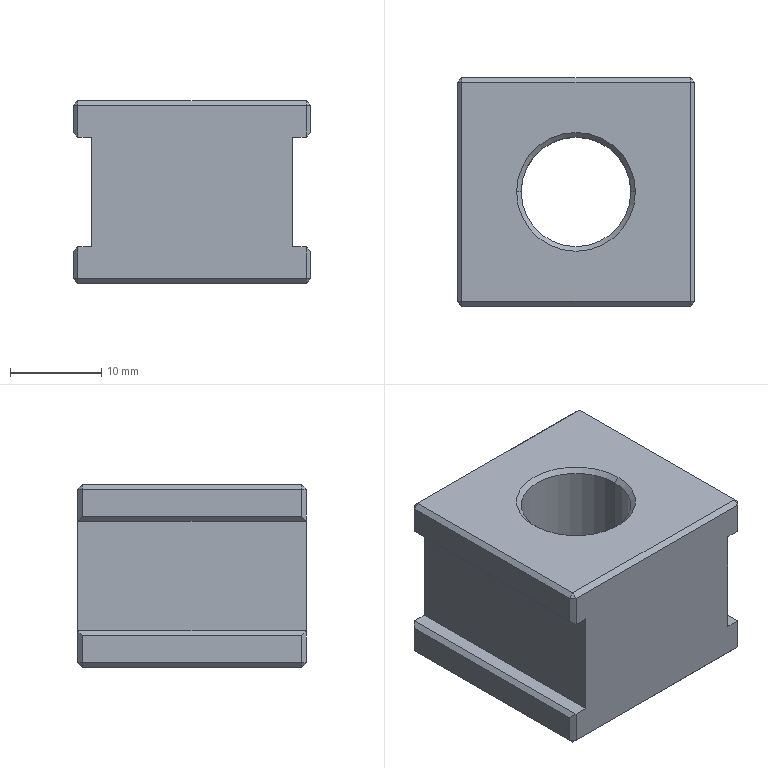Part | STEP file | MT-COMBO-119-S014 | 1 solid | 51 faces | box 26 x 25 x 20 mm | volume 9252 mm3 | plane 43 | cylinder 4 | cone 4 | commonest cylinder face diameters 10 x2 12 x2
STEP:
#1=CARTESIAN_POINT('',(0.,9.5,-15.));
#2=VERTEX_POINT('',#1);
#3=CARTESIAN_POINT('',(0.,9.5,-5.));
#4=VERTEX_POINT('',#3);
#5=CARTESIAN_POINT('',(0.,9.5,-10.));
#6=DIRECTION('',(0.,-1.,0.));
#7=DIRECTION('',(0.,0.,-1.));
#8=AXIS2_PLACEMENT_3D('',#5,#6,#7);
#9=CIRCLE('',#8,5.);
#10=EDGE_CURVE('',#2,#4,#9,.T.);
#11=ORIENTED_EDGE('',*,*,#10,.T.);
#12=CARTESIAN_POINT('',(0.,12.5,-5.));
#13=VERTEX_POINT('',#12);
#14=CARTESIAN_POINT('',(0.,9.5,-5.));
#15=DIRECTION('',(0.,1.,0.));
#16=VECTOR('',#15,1000.);
#17=LINE('',#14,#16);
#18=EDGE_CURVE('',#4,#13,#17,.T.);
#19=ORIENTED_EDGE('',*,*,#18,.T.);
#20=CARTESIAN_POINT('',(0.,12.5,-15.));
#21=VERTEX_POINT('',#20);
#22=CARTESIAN_POINT('',(0.,12.5,-10.));
#23=DIRECTION('',(0.,-1.,0.));
#24=DIRECTION('',(0.,0.,-1.));
#25=AXIS2_PLACEMENT_3D('',#22,#23,#24);
#26=CIRCLE('',#25,5.);
#27=EDGE_CURVE('',#21,#13,#26,.T.);
#28=ORIENTED_EDGE('',*,*,#27,.F.);
#29=CARTESIAN_POINT('',(0.,9.5,-15.));
#30=DIRECTION('',(0.,1.,0.));
#31=VECTOR('',#30,1000.);
#32=LINE('',#29,#31);
#33=EDGE_CURVE('',#2,#21,#32,.T.);
#34=ORIENTED_EDGE('',*,*,#33,.F.);
#35=EDGE_LOOP('',(#11,#19,#28,#34));
#36=FACE_OUTER_BOUND('',#35,.T.);
#37=CARTESIAN_POINT('',(0.,9.5,-10.));
#38=DIRECTION('',(0.,1.,0.));
#39=DIRECTION('',(0.,0.,-1.));
#40=AXIS2_PLACEMENT_3D('',#37,#38,#39);
#41=CYLINDRICAL_SURFACE('',#40,5.);
#42=ADVANCED_FACE('',(#36),#41,.F.);
#43=CARTESIAN_POINT('',(-6.,0.,-0.5));
#44=VERTEX_POINT('',#43);
#45=CARTESIAN_POINT('',(6.,0.,-0.5));
#46=VERTEX_POINT('',#45);
#47=CARTESIAN_POINT('',(0.,0.,-0.5));
#48=DIRECTION('',(0.,0.,-1.));
#49=DIRECTION('',(1.,0.,0.));
#50=AXIS2_PLACEMENT_3D('',#47,#48,#49);
#51=CIRCLE('',#50,6.);
#52=EDGE_CURVE('',#44,#46,#51,.T.);
#53=ORIENTED_EDGE('',*,*,#52,.T.);
#54=CARTESIAN_POINT('',(6.5,0.,0.));
#55=VERTEX_POINT('',#54);
#56=CARTESIAN_POINT('',(6.5,0.,0.));
#57=DIRECTION('',(0.7071,0.,0.7071));
#58=VECTOR('',#57,1000.);
#59=LINE('',#56,#58);
#60=EDGE_CURVE('',#46,#55,#59,.T.);
#61=ORIENTED_EDGE('',*,*,#60,.T.);
#62=CARTESIAN_POINT('',(-6.5,0.,0.));
#63=VERTEX_POINT('',#62);
#64=CARTESIAN_POINT('',(0.,0.,0.));
#65=DIRECTION('',(0.,0.,1.));
#66=DIRECTION('',(1.,0.,0.));
#67=AXIS2_PLACEMENT_3D('',#64,#65,#66);
#68=CIRCLE('',#67,6.5);
#69=EDGE_CURVE('',#55,#63,#68,.T.);
#70=ORIENTED_EDGE('',*,*,#69,.T.);
#71=CARTESIAN_POINT('',(-6.5,0.,0.));
#72=DIRECTION('',(-0.7071,0.,0.7071));
#73=VECTOR('',#72,1000.);
#74=LINE('',#71,#73);
#75=EDGE_CURVE('',#44,#63,#74,.T.);
#76=ORIENTED_EDGE('',*,*,#75,.F.);
#77=EDGE_LOOP('',(#53,#61,#70,#76));
#78=FACE_OUTER_BOUND('',#77,.T.);
#79=CARTESIAN_POINT('',(0.,0.,0.));
#80=DIRECTION('',(0.,0.,1.));
#81=DIRECTION('',(-1.,0.,0.));
#82=AXIS2_PLACEMENT_3D('',#79,#80,#81);
#83=CONICAL_SURFACE('',#82,6.5,0.7854);
#84=ADVANCED_FACE('',(#78),#83,.F.);
#85=CARTESIAN_POINT('',(6.,0.,-19.5));
#86=VERTEX_POINT('',#85);
#87=CARTESIAN_POINT('',(-6.,0.,-19.5));
#88=VERTEX_POINT('',#87);
#89=CARTESIAN_POINT('',(0.,0.,-19.5));
#90=DIRECTION('',(0.,0.,1.));
#91=DIRECTION('',(1.,0.,0.));
#92=AXIS2_PLACEMENT_3D('',#89,#90,#91);
#93=CIRCLE('',#92,6.);
#94=EDGE_CURVE('',#86,#88,#93,.T.);
#95=ORIENTED_EDGE('',*,*,#94,.T.);
#96=CARTESIAN_POINT('',(-6.5,0.,-20.));
#97=VERTEX_POINT('',#96);
#98=CARTESIAN_POINT('',(-6.,0.,-19.5));
#99=DIRECTION('',(-0.7071,0.,-0.7071));
#100=VECTOR('',#99,1000.);
#101=LINE('',#98,#100);
#102=EDGE_CURVE('',#88,#97,#101,.T.);
#103=ORIENTED_EDGE('',*,*,#102,.T.);
#104=CARTESIAN_POINT('',(6.5,0.,-20.));
#105=VERTEX_POINT('',#104);
#106=CARTESIAN_POINT('',(0.,0.,-20.));
#107=DIRECTION('',(0.,0.,-1.));
#108=DIRECTION('',(1.,0.,0.));
#109=AXIS2_PLACEMENT_3D('',#106,#107,#108);
#110=CIRCLE('',#109,6.5);
#111=EDGE_CURVE('',#97,#105,#110,.T.);
#112=ORIENTED_EDGE('',*,*,#111,.T.);
#113=CARTESIAN_POINT('',(6.,0.,-19.5));
#114=DIRECTION('',(0.7071,0.,-0.7071));
#115=VECTOR('',#114,1000.);
#116=LINE('',#113,#115);
#117=EDGE_CURVE('',#86,#105,#116,.T.);
#118=ORIENTED_EDGE('',*,*,#117,.F.);
#119=EDGE_LOOP('',(#95,#103,#112,#118));
#120=FACE_OUTER_BOUND('',#119,.T.);
#121=CARTESIAN_POINT('',(0.,0.,-19.5));
#122=DIRECTION('',(0.,0.,-1.));
#123=DIRECTION('',(1.,0.,0.));
#124=AXIS2_PLACEMENT_3D('',#121,#122,#123);
#125=CONICAL_SURFACE('',#124,6.,0.7854);
#126=ADVANCED_FACE('',(#120),#125,.F.);
#127=ORIENTED_EDGE('',*,*,#52,.F.);
#128=CARTESIAN_POINT('',(-6.,0.,0.));
#129=DIRECTION('',(0.,0.,-1.));
#130=VECTOR('',#129,1000.);
#131=LINE('',#128,#130);
#132=EDGE_CURVE('',#44,#88,#131,.T.);
#133=ORIENTED_EDGE('',*,*,#132,.T.);
#134=ORIENTED_EDGE('',*,*,#94,.F.);
#135=CARTESIAN_POINT('',(6.,0.,0.));
#136=DIRECTION('',(0.,0.,-1.));
#137=VECTOR('',#136,1000.);
#138=LINE('',#135,#137);
#139=EDGE_CURVE('',#46,#86,#138,.T.);
#140=ORIENTED_EDGE('',*,*,#139,.F.);
#141=EDGE_LOOP('',(#127,#133,#134,#140));
#142=FACE_OUTER_BOUND('',#141,.T.);
#143=CARTESIAN_POINT('',(0.,0.,0.));
#144=DIRECTION('',(0.,0.,-1.));
#145=DIRECTION('',(1.,0.,0.));
#146=AXIS2_PLACEMENT_3D('',#143,#144,#145);
#147=CYLINDRICAL_SURFACE('',#146,6.);
#148=ADVANCED_FACE('',(#142),#147,.F.);
#149=CARTESIAN_POINT('',(-11.,-12.5,-4.));
#150=VERTEX_POINT('',#149);
#151=CARTESIAN_POINT('',(-12.5,-12.5,-4.));
#152=VERTEX_POINT('',#151);
#153=CARTESIAN_POINT('',(13.,-12.5,-4.));
#154=DIRECTION('',(-1.,0.,0.));
#155=VECTOR('',#154,1000.);
#156=LINE('',#153,#155);
#157=EDGE_CURVE('',#150,#152,#156,.T.);
#158=ORIENTED_EDGE('',*,*,#157,.F.);
#159=CARTESIAN_POINT('',(-11.,-12.5,-16.));
#160=VERTEX_POINT('',#159);
#161=CARTESIAN_POINT('',(-11.,-12.5,-20.));
#162=DIRECTION('',(0.,0.,-1.));
#163=VECTOR('',#162,1000.);
#164=LINE('',#161,#163);
#165=EDGE_CURVE('',#150,#160,#164,.T.);
#166=ORIENTED_EDGE('',*,*,#165,.T.);
#167=CARTESIAN_POINT('',(-12.5,-12.5,-16.));
#168=VERTEX_POINT('',#167);
#169=CARTESIAN_POINT('',(13.,-12.5,-16.));
#170=DIRECTION('',(1.,0.,0.));
#171=VECTOR('',#170,1000.);
#172=LINE('',#169,#171);
#173=EDGE_CURVE('',#168,#160,#172,.T.);
#174=ORIENTED_EDGE('',*,*,#173,.F.);
#175=CARTESIAN_POINT('',(-12.5,-12.5,-19.5));
#176=VERTEX_POINT('',#175);
#177=CARTESIAN_POINT('',(-12.5,-12.5,-20.));
#178=DIRECTION('',(0.,0.,1.));
#179=VECTOR('',#178,1000.);
#180=LINE('',#177,#179);
#181=EDGE_CURVE('',#176,#168,#180,.T.);
#182=ORIENTED_EDGE('',*,*,#181,.F.);
#183=CARTESIAN_POINT('',(12.5,-12.5,-19.5));
#184=VERTEX_POINT('',#183);
#185=CARTESIAN_POINT('',(-13.,-12.5,-19.5));
#186=DIRECTION('',(-1.,0.,0.));
#187=VECTOR('',#186,1000.);
#188=LINE('',#185,#187);
#189=EDGE_CURVE('',#184,#176,#188,.T.);
#190=ORIENTED_EDGE('',*,*,#189,.F.);
#191=CARTESIAN_POINT('',(12.5,-12.5,-16.));
#192=VERTEX_POINT('',#191);
#193=CARTESIAN_POINT('',(12.5,-12.5,-20.));
#194=DIRECTION('',(0.,0.,-1.));
#195=VECTOR('',#194,1000.);
#196=LINE('',#193,#195);
#197=EDGE_CURVE('',#192,#184,#196,.T.);
#198=ORIENTED_EDGE('',*,*,#197,.F.);
#199=CARTESIAN_POINT('',(11.,-12.5,-16.));
#200=VERTEX_POINT('',#199);
#201=CARTESIAN_POINT('',(13.,-12.5,-16.));
#202=DIRECTION('',(-1.,0.,0.));
#203=VECTOR('',#202,1000.);
#204=LINE('',#201,#203);
#205=EDGE_CURVE('',#192,#200,#204,.T.);
#206=ORIENTED_EDGE('',*,*,#205,.T.);
#207=CARTESIAN_POINT('',(11.,-12.5,-4.));
#208=VERTEX_POINT('',#207);
#209=CARTESIAN_POINT('',(11.,-12.5,-20.));
#210=DIRECTION('',(0.,0.,1.));
#211=VECTOR('',#210,1000.);
#212=LINE('',#209,#211);
#213=EDGE_CURVE('',#200,#208,#212,.T.);
#214=ORIENTED_EDGE('',*,*,#213,.T.);
#215=CARTESIAN_POINT('',(12.5,-12.5,-4.));
#216=VERTEX_POINT('',#215);
#217=CARTESIAN_POINT('',(13.,-12.5,-4.));
#218=DIRECTION('',(1.,0.,0.));
#219=VECTOR('',#218,1000.);
#220=LINE('',#217,#219);
#221=EDGE_CURVE('',#208,#216,#220,.T.);
#222=ORIENTED_EDGE('',*,*,#221,.T.);
#223=CARTESIAN_POINT('',(12.5,-12.5,-0.5));
#224=VERTEX_POINT('',#223);
#225=CARTESIAN_POINT('',(12.5,-12.5,-20.));
#226=DIRECTION('',(0.,0.,-1.));
#227=VECTOR('',#226,1000.);
#228=LINE('',#225,#227);
#229=EDGE_CURVE('',#224,#216,#228,.T.);
#230=ORIENTED_EDGE('',*,*,#229,.F.);
#231=CARTESIAN_POINT('',(-12.5,-12.5,-0.5));
#232=VERTEX_POINT('',#231);
#233=CARTESIAN_POINT('',(13.,-12.5,-0.5));
#234=DIRECTION('',(1.,0.,0.));
#235=VECTOR('',#234,1000.);
#236=LINE('',#233,#235);
#237=EDGE_CURVE('',#232,#224,#236,.T.);
#238=ORIENTED_EDGE('',*,*,#237,.F.);
#239=CARTESIAN_POINT('',(-12.5,-12.5,-20.));
#240=DIRECTION('',(0.,0.,1.));
#241=VECTOR('',#240,1000.);
#242=LINE('',#239,#241);
#243=EDGE_CURVE('',#152,#232,#242,.T.);
#244=ORIENTED_EDGE('',*,*,#243,.F.);
#245=EDGE_LOOP('',(#158,#166,#174,#182,#190,#198,#206,#214,#222,#230,#238,#244));
#246=FACE_OUTER_BOUND('',#245,.T.);
#247=CARTESIAN_POINT('',(13.,-12.5,-20.));
#248=DIRECTION('',(0.,1.,0.));
#249=DIRECTION('',(0.,0.,-1.));
#250=AXIS2_PLACEMENT_3D('',#247,#248,#249);
#251=PLANE('',#250);
#252=ADVANCED_FACE('',(#246),#251,.F.);
#253=CARTESIAN_POINT('',(13.,12.,-19.5));
#254=VERTEX_POINT('',#253);
#255=CARTESIAN_POINT('',(13.,-12.,-19.5));
#256=VERTEX_POINT('',#255);
#257=CARTESIAN_POINT('',(13.,-12.5,-19.5));
#258=DIRECTION('',(0.,-1.,0.));
#259=VECTOR('',#258,1000.);
#260=LINE('',#257,#259);
#261=EDGE_CURVE('',#254,#256,#260,.T.);
#262=ORIENTED_EDGE('',*,*,#261,.F.);
#263=CARTESIAN_POINT('',(13.,12.,-16.5));
#264=VERTEX_POINT('',#263);
#265=CARTESIAN_POINT('',(13.,12.,-20.));
#266=DIRECTION('',(0.,0.,-1.));
#267=VECTOR('',#266,1000.);
#268=LINE('',#265,#267);
#269=EDGE_CURVE('',#264,#254,#268,.T.);
#270=ORIENTED_EDGE('',*,*,#269,.F.);
#271=CARTESIAN_POINT('',(13.,-12.,-16.5));
#272=VERTEX_POINT('',#271);
#273=CARTESIAN_POINT('',(13.,12.5,-16.5));
#274=DIRECTION('',(0.,1.,0.));
#275=VECTOR('',#274,1000.);
#276=LINE('',#273,#275);
#277=EDGE_CURVE('',#272,#264,#276,.T.);
#278=ORIENTED_EDGE('',*,*,#277,.F.);
#279=CARTESIAN_POINT('',(13.,-12.,-20.));
#280=DIRECTION('',(0.,0.,1.));
#281=VECTOR('',#280,1000.);
#282=LINE('',#279,#281);
#283=EDGE_CURVE('',#256,#272,#282,.T.);
#284=ORIENTED_EDGE('',*,*,#283,.F.);
#285=EDGE_LOOP('',(#262,#270,#278,#284));
#286=FACE_OUTER_BOUND('',#285,.T.);
#287=CARTESIAN_POINT('',(13.,-12.5,-20.));
#288=DIRECTION('',(-1.,0.,0.));
#289=DIRECTION('',(0.,0.,-1.));
#290=AXIS2_PLACEMENT_3D('',#287,#288,#289);
#291=PLANE('',#290);
#292=ADVANCED_FACE('',(#286),#291,.F.);
#293=CARTESIAN_POINT('',(13.,-12.,-0.5));
#294=VERTEX_POINT('',#293);
#295=CARTESIAN_POINT('',(13.,12.,-0.5));
#296=VERTEX_POINT('',#295);
#297=CARTESIAN_POINT('',(13.,-12.5,-0.5));
#298=DIRECTION('',(0.,1.,0.));
#299=VECTOR('',#298,1000.);
#300=LINE('',#297,#299);
#301=EDGE_CURVE('',#294,#296,#300,.T.);
#302=ORIENTED_EDGE('',*,*,#301,.F.);
#303=CARTESIAN_POINT('',(13.,-12.,-3.5));
#304=VERTEX_POINT('',#303);
#305=CARTESIAN_POINT('',(13.,-12.,-20.));
#306=DIRECTION('',(0.,0.,1.));
#307=VECTOR('',#306,1000.);
#308=LINE('',#305,#307);
#309=EDGE_CURVE('',#304,#294,#308,.T.);
#310=ORIENTED_EDGE('',*,*,#309,.F.);
#311=CARTESIAN_POINT('',(13.,12.,-3.5));
#312=VERTEX_POINT('',#311);
#313=CARTESIAN_POINT('',(13.,-12.5,-3.5));
#314=DIRECTION('',(0.,-1.,0.));
#315=VECTOR('',#314,1000.);
#316=LINE('',#313,#315);
#317=EDGE_CURVE('',#312,#304,#316,.T.);
#318=ORIENTED_EDGE('',*,*,#317,.F.);
#319=CARTESIAN_POINT('',(13.,12.,-20.));
#320=DIRECTION('',(0.,0.,-1.));
#321=VECTOR('',#320,1000.);
#322=LINE('',#319,#321);
#323=EDGE_CURVE('',#296,#312,#322,.T.);
#324=ORIENTED_EDGE('',*,*,#323,.F.);
#325=EDGE_LOOP('',(#302,#310,#318,#324));
#326=FACE_OUTER_BOUND('',#325,.T.);
#327=CARTESIAN_POINT('',(13.,-12.5,-20.));
#328=DIRECTION('',(-1.,0.,0.));
#329=DIRECTION('',(0.,0.,-1.));
#330=AXIS2_PLACEMENT_3D('',#327,#328,#329);
#331=PLANE('',#330);
#332=ADVANCED_FACE('',(#326),#331,.F.);
#333=ORIENTED_EDGE('',*,*,#27,.T.);
#334=CARTESIAN_POINT('',(0.,12.5,-10.));
#335=DIRECTION('',(0.,-1.,0.));
#336=DIRECTION('',(0.,0.,-1.));
#337=AXIS2_PLACEMENT_3D('',#334,#335,#336);
#338=CIRCLE('',#337,5.);
#339=EDGE_CURVE('',#13,#21,#338,.T.);
#340=ORIENTED_EDGE('',*,*,#339,.T.);
#341=EDGE_LOOP('',(#333,#340));
#342=FACE_BOUND('',#341,.T.);
#343=CARTESIAN_POINT('',(12.5,12.5,-0.5));
#344=VERTEX_POINT('',#343);
#345=CARTESIAN_POINT('',(-12.5,12.5,-0.5));
#346=VERTEX_POINT('',#345);
#347=CARTESIAN_POINT('',(13.,12.5,-0.5));
#348=DIRECTION('',(-1.,0.,0.));
#349=VECTOR('',#348,1000.);
#350=LINE('',#347,#349);
#351=EDGE_CURVE('',#344,#346,#350,.T.);
#352=ORIENTED_EDGE('',*,*,#351,.F.);
#353=CARTESIAN_POINT('',(12.5,12.5,-4.));
#354=VERTEX_POINT('',#353);
#355=CARTESIAN_POINT('',(12.5,12.5,-20.));
#356=DIRECTION('',(0.,0.,1.));
#357=VECTOR('',#356,1000.);
#358=LINE('',#355,#357);
#359=EDGE_CURVE('',#354,#344,#358,.T.);
#360=ORIENTED_EDGE('',*,*,#359,.F.);
#361=CARTESIAN_POINT('',(11.,12.5,-4.));
#362=VERTEX_POINT('',#361);
#363=CARTESIAN_POINT('',(13.,12.5,-4.));
#364=DIRECTION('',(-1.,0.,0.));
#365=VECTOR('',#364,1000.);
#366=LINE('',#363,#365);
#367=EDGE_CURVE('',#354,#362,#366,.T.);
#368=ORIENTED_EDGE('',*,*,#367,.T.);
#369=CARTESIAN_POINT('',(11.,12.5,-16.));
#370=VERTEX_POINT('',#369);
#371=CARTESIAN_POINT('',(11.,12.5,-20.));
#372=DIRECTION('',(0.,0.,-1.));
#373=VECTOR('',#372,1000.);
#374=LINE('',#371,#373);
#375=EDGE_CURVE('',#362,#370,#374,.T.);
#376=ORIENTED_EDGE('',*,*,#375,.T.);
#377=CARTESIAN_POINT('',(12.5,12.5,-16.));
#378=VERTEX_POINT('',#377);
#379=CARTESIAN_POINT('',(13.,12.5,-16.));
#380=DIRECTION('',(1.,0.,0.));
#381=VECTOR('',#380,1000.);
#382=LINE('',#379,#381);
#383=EDGE_CURVE('',#370,#378,#382,.T.);
#384=ORIENTED_EDGE('',*,*,#383,.T.);
#385=CARTESIAN_POINT('',(12.5,12.5,-19.5));
#386=VERTEX_POINT('',#385);
#387=CARTESIAN_POINT('',(12.5,12.5,-20.));
#388=DIRECTION('',(0.,0.,1.));
#389=VECTOR('',#388,1000.);
#390=LINE('',#387,#389);
#391=EDGE_CURVE('',#386,#378,#390,.T.);
#392=ORIENTED_EDGE('',*,*,#391,.F.);
#393=CARTESIAN_POINT('',(-12.5,12.5,-19.5));
#394=VERTEX_POINT('',#393);
#395=CARTESIAN_POINT('',(13.,12.5,-19.5));
#396=DIRECTION('',(1.,0.,0.));
#397=VECTOR('',#396,1000.);
#398=LINE('',#395,#397);
#399=EDGE_CURVE('',#394,#386,#398,.T.);
#400=ORIENTED_EDGE('',*,*,#399,.F.);
#401=CARTESIAN_POINT('',(-12.5,12.5,-16.));
#402=VERTEX_POINT('',#401);
#403=CARTESIAN_POINT('',(-12.5,12.5,-20.));
#404=DIRECTION('',(0.,0.,-1.));
#405=VECTOR('',#404,1000.);
#406=LINE('',#403,#405);
#407=EDGE_CURVE('',#402,#394,#406,.T.);
#408=ORIENTED_EDGE('',*,*,#407,.F.);
#409=CARTESIAN_POINT('',(-11.,12.5,-16.));
#410=VERTEX_POINT('',#409);
#411=CARTESIAN_POINT('',(13.,12.5,-16.));
#412=DIRECTION('',(-1.,0.,0.));
#413=VECTOR('',#412,1000.);
#414=LINE('',#411,#413);
#415=EDGE_CURVE('',#410,#402,#414,.T.);
#416=ORIENTED_EDGE('',*,*,#415,.F.);
#417=CARTESIAN_POINT('',(-11.,12.5,-4.));
#418=VERTEX_POINT('',#417);
#419=CARTESIAN_POINT('',(-11.,12.5,-20.));
#420=DIRECTION('',(0.,0.,1.));
#421=VECTOR('',#420,1000.);
#422=LINE('',#419,#421);
#423=EDGE_CURVE('',#410,#418,#422,.T.);
#424=ORIENTED_EDGE('',*,*,#423,.T.);
#425=CARTESIAN_POINT('',(-12.5,12.5,-4.));
#426=VERTEX_POINT('',#425);
#427=CARTESIAN_POINT('',(13.,12.5,-4.));
#428=DIRECTION('',(1.,0.,0.));
#429=VECTOR('',#428,1000.);
#430=LINE('',#427,#429);
#431=EDGE_CURVE('',#426,#418,#430,.T.);
#432=ORIENTED_EDGE('',*,*,#431,.F.);
#433=CARTESIAN_POINT('',(-12.5,12.5,-20.));
#434=DIRECTION('',(0.,0.,-1.));
#435=VECTOR('',#434,1000.);
#436=LINE('',#433,#435);
#437=EDGE_CURVE('',#346,#426,#436,.T.);
#438=ORIENTED_EDGE('',*,*,#437,.F.);
#439=EDGE_LOOP('',(#352,#360,#368,#376,#384,#392,#400,#408,#416,#424,#432,#438));
#440=FACE_OUTER_BOUND('',#439,.T.);
#441=CARTESIAN_POINT('',(13.,12.5,-20.));
#442=DIRECTION('',(0.,-1.,0.));
#443=DIRECTION('',(0.,0.,1.));
#444=AXIS2_PLACEMENT_3D('',#441,#442,#443);
#445=PLANE('',#444);
#446=ADVANCED_FACE('',(#342,#440),#445,.F.);
#447=CARTESIAN_POINT('',(-13.,12.,-16.5));
#448=VERTEX_POINT('',#447);
#449=CARTESIAN_POINT('',(-13.,-12.,-16.5));
#450=VERTEX_POINT('',#449);
#451=CARTESIAN_POINT('',(-13.,-12.5,-16.5));
#452=DIRECTION('',(0.,-1.,0.));
#453=VECTOR('',#452,1000.);
#454=LINE('',#451,#453);
#455=EDGE_CURVE('',#448,#450,#454,.T.);
#456=ORIENTED_EDGE('',*,*,#455,.F.);
#457=CARTESIAN_POINT('',(-13.,12.,-19.5));
#458=VERTEX_POINT('',#457);
#459=CARTESIAN_POINT('',(-13.,12.,-20.));
#460=DIRECTION('',(0.,0.,1.));
#461=VECTOR('',#460,1000.);
#462=LINE('',#459,#461);
#463=EDGE_CURVE('',#458,#448,#462,.T.);
#464=ORIENTED_EDGE('',*,*,#463,.F.);
#465=CARTESIAN_POINT('',(-13.,-12.,-19.5));
#466=VERTEX_POINT('',#465);
#467=CARTESIAN_POINT('',(-13.,12.5,-19.5));
#468=DIRECTION('',(0.,1.,0.));
#469=VECTOR('',#468,1000.);
#470=LINE('',#467,#469);
#471=EDGE_CURVE('',#466,#458,#470,.T.);
#472=ORIENTED_EDGE('',*,*,#471,.F.);
#473=CARTESIAN_POINT('',(-13.,-12.,-20.));
#474=DIRECTION('',(0.,0.,-1.));
#475=VECTOR('',#474,1000.);
#476=LINE('',#473,#475);
#477=EDGE_CURVE('',#450,#466,#476,.T.);
#478=ORIENTED_EDGE('',*,*,#477,.F.);
#479=EDGE_LOOP('',(#456,#464,#472,#478));
#480=FACE_OUTER_BOUND('',#479,.T.);
#481=CARTESIAN_POINT('',(-13.,-12.5,-20.));
#482=DIRECTION('',(1.,0.,0.));
#483=DIRECTION('',(0.,0.,1.));
#484=AXIS2_PLACEMENT_3D('',#481,#482,#483);
#485=PLANE('',#484);
#486=ADVANCED_FACE('',(#480),#485,.F.);
#487=CARTESIAN_POINT('',(-13.,-12.,-3.5));
#488=VERTEX_POINT('',#487);
#489=CARTESIAN_POINT('',(-13.,12.,-3.5));
#490=VERTEX_POINT('',#489);
#491=CARTESIAN_POINT('',(-13.,-12.5,-3.5));
#492=DIRECTION('',(0.,1.,0.));
#493=VECTOR('',#492,1000.);
#494=LINE('',#491,#493);
#495=EDGE_CURVE('',#488,#490,#494,.T.);
#496=ORIENTED_EDGE('',*,*,#495,.F.);
#497=CARTESIAN_POINT('',(-13.,-12.,-0.5));
#498=VERTEX_POINT('',#497);
#499=CARTESIAN_POINT('',(-13.,-12.,-20.));
#500=DIRECTION('',(0.,0.,-1.));
#501=VECTOR('',#500,1000.);
#502=LINE('',#499,#501);
#503=EDGE_CURVE('',#498,#488,#502,.T.);
#504=ORIENTED_EDGE('',*,*,#503,.F.);
#505=CARTESIAN_POINT('',(-13.,12.,-0.5));
#506=VERTEX_POINT('',#505);
#507=CARTESIAN_POINT('',(-13.,-12.5,-0.5));
#508=DIRECTION('',(0.,-1.,0.));
#509=VECTOR('',#508,1000.);
#510=LINE('',#507,#509);
#511=EDGE_CURVE('',#506,#498,#510,.T.);
#512=ORIENTED_EDGE('',*,*,#511,.F.);
#513=CARTESIAN_POINT('',(-13.,12.,-20.));
#514=DIRECTION('',(0.,0.,1.));
#515=VECTOR('',#514,1000.);
#516=LINE('',#513,#515);
#517=EDGE_CURVE('',#490,#506,#516,.T.);
#518=ORIENTED_EDGE('',*,*,#517,.F.);
#519=EDGE_LOOP('',(#496,#504,#512,#518));
#520=FACE_OUTER_BOUND('',#519,.T.);
#521=CARTESIAN_POINT('',(-13.,-12.5,-20.));
#522=DIRECTION('',(1.,0.,0.));
#523=DIRECTION('',(0.,0.,1.));
#524=AXIS2_PLACEMENT_3D('',#521,#522,#523);
#525=PLANE('',#524);
#526=ADVANCED_FACE('',(#520),#525,.F.);
#527=CARTESIAN_POINT('',(0.,0.,-20.));
#528=DIRECTION('',(0.,0.,-1.));
#529=DIRECTION('',(1.,0.,0.));
#530=AXIS2_PLACEMENT_3D('',#527,#528,#529);
#531=CIRCLE('',#530,6.5);
#532=EDGE_CURVE('',#105,#97,#531,.T.);
#533=ORIENTED_EDGE('',*,*,#532,.F.);
#534=ORIENTED_EDGE('',*,*,#111,.F.);
#535=EDGE_LOOP('',(#533,#534));
#536=FACE_BOUND('',#535,.T.);
#537=CARTESIAN_POINT('',(12.5,-12.,-20.));
#538=VERTEX_POINT('',#537);
#539=CARTESIAN_POINT('',(12.5,12.,-20.));
#540=VERTEX_POINT('',#539);
#541=CARTESIAN_POINT('',(12.5,12.5,-20.));
#542=DIRECTION('',(0.,1.,0.));
#543=VECTOR('',#542,1000.);
#544=LINE('',#541,#543);
#545=EDGE_CURVE('',#538,#540,#544,.T.);
#546=ORIENTED_EDGE('',*,*,#545,.F.);
#547=CARTESIAN_POINT('',(-12.5,-12.,-20.));
#548=VERTEX_POINT('',#547);
#549=CARTESIAN_POINT('',(13.,-12.,-20.));
#550=DIRECTION('',(1.,0.,0.));
#551=VECTOR('',#550,1000.);
#552=LINE('',#549,#551);
#553=EDGE_CURVE('',#548,#538,#552,.T.);
#554=ORIENTED_EDGE('',*,*,#553,.F.);
#555=CARTESIAN_POINT('',(-12.5,12.,-20.));
#556=VERTEX_POINT('',#555);
#557=CARTESIAN_POINT('',(-12.5,-12.5,-20.));
#558=DIRECTION('',(0.,-1.,0.));
#559=VECTOR('',#558,1000.);
#560=LINE('',#557,#559);
#561=EDGE_CURVE('',#556,#548,#560,.T.);
#562=ORIENTED_EDGE('',*,*,#561,.F.);
#563=CARTESIAN_POINT('',(-13.,12.,-20.));
#564=DIRECTION('',(-1.,0.,0.));
#565=VECTOR('',#564,1000.);
#566=LINE('',#563,#565);
#567=EDGE_CURVE('',#540,#556,#566,.T.);
#568=ORIENTED_EDGE('',*,*,#567,.F.);
#569=EDGE_LOOP('',(#546,#554,#562,#568));
#570=FACE_OUTER_BOUND('',#569,.T.);
#571=CARTESIAN_POINT('',(0.,0.,-20.));
#572=DIRECTION('',(0.,0.,-1.));
#573=DIRECTION('',(1.,0.,0.));
#574=AXIS2_PLACEMENT_3D('',#571,#572,#573);
#575=PLANE('',#574);
#576=ADVANCED_FACE('',(#536,#570),#575,.T.);
#577=CARTESIAN_POINT('',(0.,0.,0.));
#578=DIRECTION('',(0.,0.,1.));
#579=DIRECTION('',(1.,0.,0.));
#580=AXIS2_PLACEMENT_3D('',#577,#578,#579);
#581=CIRCLE('',#580,6.5);
#582=EDGE_CURVE('',#63,#55,#581,.T.);
#583=ORIENTED_EDGE('',*,*,#582,.F.);
#584=ORIENTED_EDGE('',*,*,#69,.F.);
#585=EDGE_LOOP('',(#583,#584));
#586=FACE_BOUND('',#585,.T.);
#587=CARTESIAN_POINT('',(12.5,12.,0.));
#588=VERTEX_POINT('',#587);
#589=CARTESIAN_POINT('',(12.5,-12.,0.));
#590=VERTEX_POINT('',#589);
#591=CARTESIAN_POINT('',(12.5,0.,0.));
#592=DIRECTION('',(0.,-1.,0.));
#593=VECTOR('',#592,1000.);
#594=LINE('',#591,#593);
#595=EDGE_CURVE('',#588,#590,#594,.T.);
#596=ORIENTED_EDGE('',*,*,#595,.F.);
#597=CARTESIAN_POINT('',(-12.5,12.,0.));
#598=VERTEX_POINT('',#597);
#599=CARTESIAN_POINT('',(0.,12.,0.));
#600=DIRECTION('',(1.,0.,0.));
#601=VECTOR('',#600,1000.);
#602=LINE('',#599,#601);
#603=EDGE_CURVE('',#598,#588,#602,.T.);
#604=ORIENTED_EDGE('',*,*,#603,.F.);
#605=CARTESIAN_POINT('',(-12.5,-12.,0.));
#606=VERTEX_POINT('',#605);
#607=CARTESIAN_POINT('',(-12.5,0.,0.));
#608=DIRECTION('',(0.,1.,0.));
#609=VECTOR('',#608,1000.);
#610=LINE('',#607,#609);
#611=EDGE_CURVE('',#606,#598,#610,.T.);
#612=ORIENTED_EDGE('',*,*,#611,.F.);
#613=CARTESIAN_POINT('',(0.,-12.,0.));
#614=DIRECTION('',(-1.,0.,0.));
#615=VECTOR('',#614,1000.);
#616=LINE('',#613,#615);
#617=EDGE_CURVE('',#590,#606,#616,.T.);
#618=ORIENTED_EDGE('',*,*,#617,.F.);
#619=EDGE_LOOP('',(#596,#604,#612,#618));
#620=FACE_OUTER_BOUND('',#619,.T.);
#621=CARTESIAN_POINT('',(0.,0.,0.));
#622=DIRECTION('',(0.,0.,-1.));
#623=DIRECTION('',(1.,0.,0.));
#624=AXIS2_PLACEMENT_3D('',#621,#622,#623);
#625=PLANE('',#624);
#626=ADVANCED_FACE('',(#586,#620),#625,.F.);
#627=ORIENTED_EDGE('',*,*,#132,.F.);
#628=CARTESIAN_POINT('',(0.,0.,-0.5));
#629=DIRECTION('',(0.,0.,-1.));
#630=DIRECTION('',(1.,0.,0.));
#631=AXIS2_PLACEMENT_3D('',#628,#629,#630);
#632=CIRCLE('',#631,6.);
#633=EDGE_CURVE('',#46,#44,#632,.T.);
#634=ORIENTED_EDGE('',*,*,#633,.F.);
#635=ORIENTED_EDGE('',*,*,#139,.T.);
#636=CARTESIAN_POINT('',(0.,0.,-19.5));
#637=DIRECTION('',(0.,0.,1.));
#638=DIRECTION('',(1.,0.,0.));
#639=AXIS2_PLACEMENT_3D('',#636,#637,#638);
#640=CIRCLE('',#639,6.);
#641=EDGE_CURVE('',#88,#86,#640,.T.);
#642=ORIENTED_EDGE('',*,*,#641,.F.);
#643=EDGE_LOOP('',(#627,#634,#635,#642));
#644=FACE_OUTER_BOUND('',#643,.T.);
#645=CARTESIAN_POINT('',(0.,0.,0.));
#646=DIRECTION('',(0.,0.,-1.));
#647=DIRECTION('',(1.,0.,0.));
#648=AXIS2_PLACEMENT_3D('',#645,#646,#647);
#649=CYLINDRICAL_SURFACE('',#648,6.);
#650=ADVANCED_FACE('',(#644),#649,.F.);
#651=ORIENTED_EDGE('',*,*,#173,.T.);
#652=CARTESIAN_POINT('',(-11.,13.437,-16.));
#653=DIRECTION('',(0.,1.,0.));
#654=VECTOR('',#653,1000.);
#655=LINE('',#652,#654);
#656=EDGE_CURVE('',#160,#410,#655,.T.);
#657=ORIENTED_EDGE('',*,*,#656,.T.);
#658=ORIENTED_EDGE('',*,*,#415,.T.);
#659=CARTESIAN_POINT('',(-12.5,13.437,-16.));
#660=DIRECTION('',(0.,1.,0.));
#661=VECTOR('',#660,1000.);
#662=LINE('',#659,#661);
#663=EDGE_CURVE('',#168,#402,#662,.T.);
#664=ORIENTED_EDGE('',*,*,#663,.F.);
#665=EDGE_LOOP('',(#651,#657,#658,#664));
#666=FACE_OUTER_BOUND('',#665,.T.);
#667=CARTESIAN_POINT('',(-11.,13.437,-16.));
#668=DIRECTION('',(0.,0.,-1.));
#669=DIRECTION('',(1.,0.,0.));
#670=AXIS2_PLACEMENT_3D('',#667,#668,#669);
#671=PLANE('',#670);
#672=ADVANCED_FACE('',(#666),#671,.F.);
#673=ORIENTED_EDGE('',*,*,#431,.T.);
#674=CARTESIAN_POINT('',(-11.,13.437,-4.));
#675=DIRECTION('',(0.,-1.,0.));
#676=VECTOR('',#675,1000.);
#677=LINE('',#674,#676);
#678=EDGE_CURVE('',#418,#150,#677,.T.);
#679=ORIENTED_EDGE('',*,*,#678,.T.);
#680=ORIENTED_EDGE('',*,*,#157,.T.);
#681=CARTESIAN_POINT('',(-12.5,13.437,-4.));
#682=DIRECTION('',(0.,-1.,0.));
#683=VECTOR('',#682,1000.);
#684=LINE('',#681,#683);
#685=EDGE_CURVE('',#426,#152,#684,.T.);
#686=ORIENTED_EDGE('',*,*,#685,.F.);
#687=EDGE_LOOP('',(#673,#679,#680,#686));
#688=FACE_OUTER_BOUND('',#687,.T.);
#689=CARTESIAN_POINT('',(-11.,13.437,-4.));
#690=DIRECTION('',(0.,0.,1.));
#691=DIRECTION('',(-1.,0.,0.));
#692=AXIS2_PLACEMENT_3D('',#689,#690,#691);
#693=PLANE('',#692);
#694=ADVANCED_FACE('',(#688),#693,.F.);
#695=ORIENTED_EDGE('',*,*,#165,.F.);
#696=ORIENTED_EDGE('',*,*,#678,.F.);
#697=ORIENTED_EDGE('',*,*,#423,.F.);
#698=ORIENTED_EDGE('',*,*,#656,.F.);
#699=EDGE_LOOP('',(#695,#696,#697,#698));
#700=FACE_OUTER_BOUND('',#699,.T.);
#701=CARTESIAN_POINT('',(-11.,0.,0.));
#702=DIRECTION('',(-1.,0.,0.));
#703=DIRECTION('',(0.,0.,-1.));
#704=AXIS2_PLACEMENT_3D('',#701,#702,#703);
#705=PLANE('',#704);
#706=ADVANCED_FACE('',(#700),#705,.T.);
#707=ORIENTED_EDGE('',*,*,#383,.F.);
#708=CARTESIAN_POINT('',(11.,13.437,-16.));
#709=DIRECTION('',(0.,1.,0.));
#710=VECTOR('',#709,1000.);
#711=LINE('',#708,#710);
#712=EDGE_CURVE('',#200,#370,#711,.T.);
#713=ORIENTED_EDGE('',*,*,#712,.F.);
#714=ORIENTED_EDGE('',*,*,#205,.F.);
#715=CARTESIAN_POINT('',(12.5,-12.5,-16.));
#716=DIRECTION('',(0.,-1.,0.));
#717=VECTOR('',#716,1000.);
#718=LINE('',#715,#717);
#719=EDGE_CURVE('',#378,#192,#718,.T.);
#720=ORIENTED_EDGE('',*,*,#719,.F.);
#721=EDGE_LOOP('',(#707,#713,#714,#720));
#722=FACE_OUTER_BOUND('',#721,.T.);
#723=CARTESIAN_POINT('',(11.,13.437,-16.));
#724=DIRECTION('',(0.,0.,1.));
#725=DIRECTION('',(-1.,0.,0.));
#726=AXIS2_PLACEMENT_3D('',#723,#724,#725);
#727=PLANE('',#726);
#728=ADVANCED_FACE('',(#722),#727,.T.);
#729=ORIENTED_EDGE('',*,*,#221,.F.);
#730=CARTESIAN_POINT('',(11.,13.437,-4.));
#731=DIRECTION('',(0.,-1.,0.));
#732=VECTOR('',#731,1000.);
#733=LINE('',#730,#732);
#734=EDGE_CURVE('',#362,#208,#733,.T.);
#735=ORIENTED_EDGE('',*,*,#734,.F.);
#736=ORIENTED_EDGE('',*,*,#367,.F.);
#737=CARTESIAN_POINT('',(12.5,12.5,-4.));
#738=DIRECTION('',(0.,1.,0.));
#739=VECTOR('',#738,1000.);
#740=LINE('',#737,#739);
#741=EDGE_CURVE('',#216,#354,#740,.T.);
#742=ORIENTED_EDGE('',*,*,#741,.F.);
#743=EDGE_LOOP('',(#729,#735,#736,#742));
#744=FACE_OUTER_BOUND('',#743,.T.);
#745=CARTESIAN_POINT('',(11.,13.437,-4.));
#746=DIRECTION('',(0.,0.,-1.));
#747=DIRECTION('',(1.,0.,0.));
#748=AXIS2_PLACEMENT_3D('',#745,#746,#747);
#749=PLANE('',#748);
#750=ADVANCED_FACE('',(#744),#749,.T.);
#751=ORIENTED_EDGE('',*,*,#213,.F.);
#752=ORIENTED_EDGE('',*,*,#712,.T.);
#753=ORIENTED_EDGE('',*,*,#375,.F.);
#754=ORIENTED_EDGE('',*,*,#734,.T.);
#755=EDGE_LOOP('',(#751,#752,#753,#754));
#756=FACE_OUTER_BOUND('',#755,.T.);
#757=CARTESIAN_POINT('',(11.,0.,0.));
#758=DIRECTION('',(1.,0.,0.));
#759=DIRECTION('',(0.,0.,-1.));
#760=AXIS2_PLACEMENT_3D('',#757,#758,#759);
#761=PLANE('',#760);
#762=ADVANCED_FACE('',(#756),#761,.T.);
#763=ORIENTED_EDGE('',*,*,#102,.F.);
#764=ORIENTED_EDGE('',*,*,#641,.T.);
#765=ORIENTED_EDGE('',*,*,#117,.T.);
#766=ORIENTED_EDGE('',*,*,#532,.T.);
#767=EDGE_LOOP('',(#763,#764,#765,#766));
#768=FACE_OUTER_BOUND('',#767,.T.);
#769=CARTESIAN_POINT('',(0.,0.,-19.5));
#770=DIRECTION('',(0.,0.,-1.));
#771=DIRECTION('',(1.,0.,0.));
#772=AXIS2_PLACEMENT_3D('',#769,#770,#771);
#773=CONICAL_SURFACE('',#772,6.,0.7854);
#774=ADVANCED_FACE('',(#768),#773,.F.);
#775=ORIENTED_EDGE('',*,*,#60,.F.);
#776=ORIENTED_EDGE('',*,*,#633,.T.);
#777=ORIENTED_EDGE('',*,*,#75,.T.);
#778=ORIENTED_EDGE('',*,*,#582,.T.);
#779=EDGE_LOOP('',(#775,#776,#777,#778));
#780=FACE_OUTER_BOUND('',#779,.T.);
#781=CARTESIAN_POINT('',(0.,0.,0.));
#782=DIRECTION('',(0.,0.,1.));
#783=DIRECTION('',(-1.,0.,0.));
#784=AXIS2_PLACEMENT_3D('',#781,#782,#783);
#785=CONICAL_SURFACE('',#784,6.5,0.7854);
#786=ADVANCED_FACE('',(#780),#785,.F.);
#787=CARTESIAN_POINT('',(12.5,-12.5,-0.5));
#788=DIRECTION('',(-0.7071,-0.7071,0.));
#789=VECTOR('',#788,1000.);
#790=LINE('',#787,#789);
#791=EDGE_CURVE('',#294,#224,#790,.T.);
#792=ORIENTED_EDGE('',*,*,#791,.T.);
#793=ORIENTED_EDGE('',*,*,#229,.T.);
#794=CARTESIAN_POINT('',(12.833,-12.167,-3.667));
#795=DIRECTION('',(0.5774,0.5774,0.5774));
#796=VECTOR('',#795,1000.);
#797=LINE('',#794,#796);
#798=EDGE_CURVE('',#216,#304,#797,.T.);
#799=ORIENTED_EDGE('',*,*,#798,.T.);
#800=ORIENTED_EDGE('',*,*,#309,.T.);
#801=EDGE_LOOP('',(#792,#793,#799,#800));
#802=FACE_OUTER_BOUND('',#801,.T.);
#803=CARTESIAN_POINT('',(13.,-12.,-20.));
#804=DIRECTION('',(-0.7071,0.7071,0.));
#805=DIRECTION('',(0.,0.,1.));
#806=AXIS2_PLACEMENT_3D('',#803,#804,#805);
#807=PLANE('',#806);
#808=ADVANCED_FACE('',(#802),#807,.F.);
#809=CARTESIAN_POINT('',(12.75,-12.,-0.25));
#810=DIRECTION('',(-0.7071,0.,0.7071));
#811=VECTOR('',#810,1000.);
#812=LINE('',#809,#811);
#813=EDGE_CURVE('',#294,#590,#812,.T.);
#814=ORIENTED_EDGE('',*,*,#813,.T.);
#815=CARTESIAN_POINT('',(12.5,-12.5,-0.5));
#816=DIRECTION('',(0.,-0.7071,-0.7071));
#817=VECTOR('',#816,1000.);
#818=LINE('',#815,#817);
#819=EDGE_CURVE('',#590,#224,#818,.T.);
#820=ORIENTED_EDGE('',*,*,#819,.T.);
#821=ORIENTED_EDGE('',*,*,#791,.F.);
#822=EDGE_LOOP('',(#814,#820,#821));
#823=FACE_OUTER_BOUND('',#822,.T.);
#824=CARTESIAN_POINT('',(12.5,-12.5,-0.5));
#825=DIRECTION('',(0.5774,-0.5774,0.5774));
#826=DIRECTION('',(0.,0.7071,0.7071));
#827=AXIS2_PLACEMENT_3D('',#824,#825,#826);
#828=PLANE('',#827);
#829=ADVANCED_FACE('',(#823),#828,.T.);
#830=ORIENTED_EDGE('',*,*,#798,.F.);
#831=ORIENTED_EDGE('',*,*,#741,.T.);
#832=CARTESIAN_POINT('',(21.167,3.833,4.667));
#833=DIRECTION('',(0.5774,-0.5774,0.5774));
#834=VECTOR('',#833,1000.);
#835=LINE('',#832,#834);
#836=EDGE_CURVE('',#354,#312,#835,.T.);
#837=ORIENTED_EDGE('',*,*,#836,.T.);
#838=ORIENTED_EDGE('',*,*,#317,.T.);
#839=EDGE_LOOP('',(#830,#831,#837,#838));
#840=FACE_OUTER_BOUND('',#839,.T.);
#841=CARTESIAN_POINT('',(13.,-12.5,-3.5));
#842=DIRECTION('',(0.7071,0.,-0.7071));
#843=DIRECTION('',(0.,1.,0.));
#844=AXIS2_PLACEMENT_3D('',#841,#842,#843);
#845=PLANE('',#844);
#846=ADVANCED_FACE('',(#840),#845,.T.);
#847=ORIENTED_EDGE('',*,*,#819,.F.);
#848=ORIENTED_EDGE('',*,*,#617,.T.);
#849=CARTESIAN_POINT('',(-12.5,-12.5,-0.5));
#850=DIRECTION('',(0.,-0.7071,-0.7071));
#851=VECTOR('',#850,1000.);
#852=LINE('',#849,#851);
#853=EDGE_CURVE('',#606,#232,#852,.T.);
#854=ORIENTED_EDGE('',*,*,#853,.T.);
#855=ORIENTED_EDGE('',*,*,#237,.T.);
#856=EDGE_LOOP('',(#847,#848,#854,#855));
#857=FACE_OUTER_BOUND('',#856,.T.);
#858=CARTESIAN_POINT('',(13.,-12.5,-0.5));
#859=DIRECTION('',(0.,0.7071,-0.7071));
#860=DIRECTION('',(1.,0.,0.));
#861=AXIS2_PLACEMENT_3D('',#858,#859,#860);
#862=PLANE('',#861);
#863=ADVANCED_FACE('',(#857),#862,.F.);
#864=ORIENTED_EDGE('',*,*,#813,.F.);
#865=ORIENTED_EDGE('',*,*,#301,.T.);
#866=CARTESIAN_POINT('',(12.5,12.,0.));
#867=DIRECTION('',(-0.7071,0.,0.7071));
#868=VECTOR('',#867,1000.);
#869=LINE('',#866,#868);
#870=EDGE_CURVE('',#296,#588,#869,.T.);
#871=ORIENTED_EDGE('',*,*,#870,.T.);
#872=ORIENTED_EDGE('',*,*,#595,.T.);
#873=EDGE_LOOP('',(#864,#865,#871,#872));
#874=FACE_OUTER_BOUND('',#873,.T.);
#875=CARTESIAN_POINT('',(13.,-12.5,-0.5));
#876=DIRECTION('',(-0.7071,0.,-0.7071));
#877=DIRECTION('',(0.,1.,0.));
#878=AXIS2_PLACEMENT_3D('',#875,#876,#877);
#879=PLANE('',#878);
#880=ADVANCED_FACE('',(#874),#879,.F.);
#881=ORIENTED_EDGE('',*,*,#836,.F.);
#882=ORIENTED_EDGE('',*,*,#359,.T.);
#883=CARTESIAN_POINT('',(12.75,12.25,-0.5));
#884=DIRECTION('',(0.7071,-0.7071,0.));
#885=VECTOR('',#884,1000.);
#886=LINE('',#883,#885);
#887=EDGE_CURVE('',#344,#296,#886,.T.);
#888=ORIENTED_EDGE('',*,*,#887,.T.);
#889=ORIENTED_EDGE('',*,*,#323,.T.);
#890=EDGE_LOOP('',(#881,#882,#888,#889));
#891=FACE_OUTER_BOUND('',#890,.T.);
#892=CARTESIAN_POINT('',(12.5,12.5,-20.));
#893=DIRECTION('',(-0.7071,-0.7071,0.));
#894=DIRECTION('',(0.,0.,1.));
#895=AXIS2_PLACEMENT_3D('',#892,#893,#894);
#896=PLANE('',#895);
#897=ADVANCED_FACE('',(#891),#896,.F.);
#898=CARTESIAN_POINT('',(-12.75,-12.,-0.25));
#899=DIRECTION('',(-0.7071,0.,-0.7071));
#900=VECTOR('',#899,1000.);
#901=LINE('',#898,#900);
#902=EDGE_CURVE('',#606,#498,#901,.T.);
#903=ORIENTED_EDGE('',*,*,#902,.T.);
#904=CARTESIAN_POINT('',(-12.5,-12.5,-0.5));
#905=DIRECTION('',(0.7071,-0.7071,0.));
#906=VECTOR('',#905,1000.);
#907=LINE('',#904,#906);
#908=EDGE_CURVE('',#498,#232,#907,.T.);
#909=ORIENTED_EDGE('',*,*,#908,.T.);
#910=ORIENTED_EDGE('',*,*,#853,.F.);
#911=EDGE_LOOP('',(#903,#909,#910));
#912=FACE_OUTER_BOUND('',#911,.T.);
#913=CARTESIAN_POINT('',(-12.5,-12.5,-0.5));
#914=DIRECTION('',(-0.5774,-0.5774,0.5774));
#915=DIRECTION('',(-0.7071,0.,-0.7071));
#916=AXIS2_PLACEMENT_3D('',#913,#914,#915);
#917=PLANE('',#916);
#918=ADVANCED_FACE('',(#912),#917,.T.);
#919=ORIENTED_EDGE('',*,*,#887,.F.);
#920=CARTESIAN_POINT('',(12.5,12.,0.));
#921=DIRECTION('',(0.,-0.7071,0.7071));
#922=VECTOR('',#921,1000.);
#923=LINE('',#920,#922);
#924=EDGE_CURVE('',#344,#588,#923,.T.);
#925=ORIENTED_EDGE('',*,*,#924,.T.);
#926=ORIENTED_EDGE('',*,*,#870,.F.);
#927=EDGE_LOOP('',(#919,#925,#926));
#928=FACE_OUTER_BOUND('',#927,.T.);
#929=CARTESIAN_POINT('',(12.5,12.,0.));
#930=DIRECTION('',(0.5774,0.5774,0.5774));
#931=DIRECTION('',(0.,0.7071,-0.7071));
#932=AXIS2_PLACEMENT_3D('',#929,#930,#931);
#933=PLANE('',#932);
#934=ADVANCED_FACE('',(#928),#933,.T.);
#935=ORIENTED_EDGE('',*,*,#908,.F.);
#936=ORIENTED_EDGE('',*,*,#503,.T.);
#937=CARTESIAN_POINT('',(-7.167,-17.833,-9.333));
#938=DIRECTION('',(0.5774,-0.5774,-0.5774));
#939=VECTOR('',#938,1000.);
#940=LINE('',#937,#939);
#941=EDGE_CURVE('',#488,#152,#940,.T.);
#942=ORIENTED_EDGE('',*,*,#941,.T.);
#943=ORIENTED_EDGE('',*,*,#243,.T.);
#944=EDGE_LOOP('',(#935,#936,#942,#943));
#945=FACE_OUTER_BOUND('',#944,.T.);
#946=CARTESIAN_POINT('',(-12.5,-12.5,-20.));
#947=DIRECTION('',(0.7071,0.7071,0.));
#948=DIRECTION('',(0.,0.,1.));
#949=AXIS2_PLACEMENT_3D('',#946,#947,#948);
#950=PLANE('',#949);
#951=ADVANCED_FACE('',(#945),#950,.F.);
#952=ORIENTED_EDGE('',*,*,#902,.F.);
#953=ORIENTED_EDGE('',*,*,#611,.T.);
#954=CARTESIAN_POINT('',(-13.,12.,-0.5));
#955=DIRECTION('',(-0.7071,0.,-0.7071));
#956=VECTOR('',#955,1000.);
#957=LINE('',#954,#956);
#958=EDGE_CURVE('',#598,#506,#957,.T.);
#959=ORIENTED_EDGE('',*,*,#958,.T.);
#960=ORIENTED_EDGE('',*,*,#511,.T.);
#961=EDGE_LOOP('',(#952,#953,#959,#960));
#962=FACE_OUTER_BOUND('',#961,.T.);
#963=CARTESIAN_POINT('',(-13.,-12.5,-0.5));
#964=DIRECTION('',(0.7071,0.,-0.7071));
#965=DIRECTION('',(0.,-1.,0.));
#966=AXIS2_PLACEMENT_3D('',#963,#964,#965);
#967=PLANE('',#966);
#968=ADVANCED_FACE('',(#962),#967,.F.);
#969=ORIENTED_EDGE('',*,*,#924,.F.);
#970=ORIENTED_EDGE('',*,*,#351,.T.);
#971=CARTESIAN_POINT('',(-12.5,12.25,-0.25));
#972=DIRECTION('',(0.,-0.7071,0.7071));
#973=VECTOR('',#972,1000.);
#974=LINE('',#971,#973);
#975=EDGE_CURVE('',#346,#598,#974,.T.);
#976=ORIENTED_EDGE('',*,*,#975,.T.);
#977=ORIENTED_EDGE('',*,*,#603,.T.);
#978=EDGE_LOOP('',(#969,#970,#976,#977));
#979=FACE_OUTER_BOUND('',#978,.T.);
#980=CARTESIAN_POINT('',(13.,12.5,-0.5));
#981=DIRECTION('',(0.,-0.7071,-0.7071));
#982=DIRECTION('',(-1.,0.,0.));
#983=AXIS2_PLACEMENT_3D('',#980,#981,#982);
#984=PLANE('',#983);
#985=ADVANCED_FACE('',(#979),#984,.F.);
#986=ORIENTED_EDGE('',*,*,#941,.F.);
#987=ORIENTED_EDGE('',*,*,#495,.T.);
#988=CARTESIAN_POINT('',(-12.188,12.812,-4.312));
#989=DIRECTION('',(0.5774,0.5774,-0.5774));
#990=VECTOR('',#989,1000.);
#991=LINE('',#988,#990);
#992=EDGE_CURVE('',#490,#426,#991,.T.);
#993=ORIENTED_EDGE('',*,*,#992,.T.);
#994=ORIENTED_EDGE('',*,*,#685,.T.);
#995=EDGE_LOOP('',(#986,#987,#993,#994));
#996=FACE_OUTER_BOUND('',#995,.T.);
#997=CARTESIAN_POINT('',(-12.5,13.437,-4.));
#998=DIRECTION('',(0.7071,0.,0.7071));
#999=DIRECTION('',(0.,-1.,0.));
#1000=AXIS2_PLACEMENT_3D('',#997,#998,#999);
#1001=PLANE('',#1000);
#1002=ADVANCED_FACE('',(#996),#1001,.F.);
#1003=ORIENTED_EDGE('',*,*,#975,.F.);
#1004=CARTESIAN_POINT('',(-13.,12.,-0.5));
#1005=DIRECTION('',(-0.7071,-0.7071,0.));
#1006=VECTOR('',#1005,1000.);
#1007=LINE('',#1004,#1006);
#1008=EDGE_CURVE('',#346,#506,#1007,.T.);
#1009=ORIENTED_EDGE('',*,*,#1008,.T.);
#1010=ORIENTED_EDGE('',*,*,#958,.F.);
#1011=EDGE_LOOP('',(#1003,#1009,#1010));
#1012=FACE_OUTER_BOUND('',#1011,.T.);
#1013=CARTESIAN_POINT('',(-13.,12.,-0.5));
#1014=DIRECTION('',(-0.5774,0.5774,0.5774));
#1015=DIRECTION('',(0.,0.7071,-0.7071));
#1016=AXIS2_PLACEMENT_3D('',#1013,#1014,#1015);
#1017=PLANE('',#1016);
#1018=ADVANCED_FACE('',(#1012),#1017,.T.);
#1019=ORIENTED_EDGE('',*,*,#992,.F.);
#1020=ORIENTED_EDGE('',*,*,#517,.T.);
#1021=ORIENTED_EDGE('',*,*,#1008,.F.);
#1022=ORIENTED_EDGE('',*,*,#437,.T.);
#1023=EDGE_LOOP('',(#1019,#1020,#1021,#1022));
#1024=FACE_OUTER_BOUND('',#1023,.T.);
#1025=CARTESIAN_POINT('',(-13.,12.,-20.));
#1026=DIRECTION('',(0.7071,-0.7071,0.));
#1027=DIRECTION('',(0.,0.,1.));
#1028=AXIS2_PLACEMENT_3D('',#1025,#1026,#1027);
#1029=PLANE('',#1028);
#1030=ADVANCED_FACE('',(#1024),#1029,.F.);
#1031=CARTESIAN_POINT('',(12.5,12.5,-19.5));
#1032=DIRECTION('',(-0.7071,0.7071,0.));
#1033=VECTOR('',#1032,1000.);
#1034=LINE('',#1031,#1033);
#1035=EDGE_CURVE('',#254,#386,#1034,.T.);
#1036=ORIENTED_EDGE('',*,*,#1035,.T.);
#1037=ORIENTED_EDGE('',*,*,#391,.T.);
#1038=CARTESIAN_POINT('',(21.167,3.833,-24.667));
#1039=DIRECTION('',(0.5774,-0.5774,-0.5774));
#1040=VECTOR('',#1039,1000.);
#1041=LINE('',#1038,#1040);
#1042=EDGE_CURVE('',#378,#264,#1041,.T.);
#1043=ORIENTED_EDGE('',*,*,#1042,.T.);
#1044=ORIENTED_EDGE('',*,*,#269,.T.);
#1045=EDGE_LOOP('',(#1036,#1037,#1043,#1044));
#1046=FACE_OUTER_BOUND('',#1045,.T.);
#1047=CARTESIAN_POINT('',(12.5,12.5,-20.));
#1048=DIRECTION('',(-0.7071,-0.7071,0.));
#1049=DIRECTION('',(0.,0.,1.));
#1050=AXIS2_PLACEMENT_3D('',#1047,#1048,#1049);
#1051=PLANE('',#1050);
#1052=ADVANCED_FACE('',(#1046),#1051,.F.);
#1053=ORIENTED_EDGE('',*,*,#1042,.F.);
#1054=ORIENTED_EDGE('',*,*,#719,.T.);
#1055=CARTESIAN_POINT('',(12.833,-12.167,-16.333));
#1056=DIRECTION('',(0.5774,0.5774,-0.5774));
#1057=VECTOR('',#1056,1000.);
#1058=LINE('',#1055,#1057);
#1059=EDGE_CURVE('',#192,#272,#1058,.T.);
#1060=ORIENTED_EDGE('',*,*,#1059,.T.);
#1061=ORIENTED_EDGE('',*,*,#277,.T.);
#1062=EDGE_LOOP('',(#1053,#1054,#1060,#1061));
#1063=FACE_OUTER_BOUND('',#1062,.T.);
#1064=CARTESIAN_POINT('',(13.,-12.5,-16.5));
#1065=DIRECTION('',(0.7071,0.,0.7071));
#1066=DIRECTION('',(0.,-1.,0.));
#1067=AXIS2_PLACEMENT_3D('',#1064,#1065,#1066);
#1068=PLANE('',#1067);
#1069=ADVANCED_FACE('',(#1063),#1068,.T.);
#1070=CARTESIAN_POINT('',(12.5,12.5,-19.5));
#1071=DIRECTION('',(0.,0.7071,0.7071));
#1072=VECTOR('',#1071,1000.);
#1073=LINE('',#1070,#1072);
#1074=EDGE_CURVE('',#540,#386,#1073,.T.);
#1075=ORIENTED_EDGE('',*,*,#1074,.T.);
#1076=ORIENTED_EDGE('',*,*,#1035,.F.);
#1077=CARTESIAN_POINT('',(12.75,12.,-19.75));
#1078=DIRECTION('',(-0.7071,0.,-0.7071));
#1079=VECTOR('',#1078,1000.);
#1080=LINE('',#1077,#1079);
#1081=EDGE_CURVE('',#254,#540,#1080,.T.);
#1082=ORIENTED_EDGE('',*,*,#1081,.T.);
#1083=EDGE_LOOP('',(#1075,#1076,#1082));
#1084=FACE_OUTER_BOUND('',#1083,.T.);
#1085=CARTESIAN_POINT('',(12.5,12.5,-19.5));
#1086=DIRECTION('',(0.5774,0.5774,-0.5774));
#1087=DIRECTION('',(0.,-0.7071,-0.7071));
#1088=AXIS2_PLACEMENT_3D('',#1085,#1086,#1087);
#1089=PLANE('',#1088);
#1090=ADVANCED_FACE('',(#1084),#1089,.T.);
#1091=ORIENTED_EDGE('',*,*,#1081,.F.);
#1092=ORIENTED_EDGE('',*,*,#261,.T.);
#1093=CARTESIAN_POINT('',(12.5,-12.,-20.));
#1094=DIRECTION('',(-0.7071,0.,-0.7071));
#1095=VECTOR('',#1094,1000.);
#1096=LINE('',#1093,#1095);
#1097=EDGE_CURVE('',#256,#538,#1096,.T.);
#1098=ORIENTED_EDGE('',*,*,#1097,.T.);
#1099=ORIENTED_EDGE('',*,*,#545,.T.);
#1100=EDGE_LOOP('',(#1091,#1092,#1098,#1099));
#1101=FACE_OUTER_BOUND('',#1100,.T.);
#1102=CARTESIAN_POINT('',(12.5,0.,-20.));
#1103=DIRECTION('',(0.7071,0.,-0.7071));
#1104=DIRECTION('',(0.,-1.,0.));
#1105=AXIS2_PLACEMENT_3D('',#1102,#1103,#1104);
#1106=PLANE('',#1105);
#1107=ADVANCED_FACE('',(#1101),#1106,.T.);
#1108=ORIENTED_EDGE('',*,*,#1059,.F.);
#1109=ORIENTED_EDGE('',*,*,#197,.T.);
#1110=CARTESIAN_POINT('',(12.75,-12.25,-19.5));
#1111=DIRECTION('',(0.7071,0.7071,0.));
#1112=VECTOR('',#1111,1000.);
#1113=LINE('',#1110,#1112);
#1114=EDGE_CURVE('',#184,#256,#1113,.T.);
#1115=ORIENTED_EDGE('',*,*,#1114,.T.);
#1116=ORIENTED_EDGE('',*,*,#283,.T.);
#1117=EDGE_LOOP('',(#1108,#1109,#1115,#1116));
#1118=FACE_OUTER_BOUND('',#1117,.T.);
#1119=CARTESIAN_POINT('',(13.,-12.,-20.));
#1120=DIRECTION('',(-0.7071,0.7071,0.));
#1121=DIRECTION('',(0.,0.,1.));
#1122=AXIS2_PLACEMENT_3D('',#1119,#1120,#1121);
#1123=PLANE('',#1122);
#1124=ADVANCED_FACE('',(#1118),#1123,.F.);
#1125=ORIENTED_EDGE('',*,*,#1074,.F.);
#1126=ORIENTED_EDGE('',*,*,#567,.T.);
#1127=CARTESIAN_POINT('',(-12.5,12.5,-19.5));
#1128=DIRECTION('',(0.,0.7071,0.7071));
#1129=VECTOR('',#1128,1000.);
#1130=LINE('',#1127,#1129);
#1131=EDGE_CURVE('',#556,#394,#1130,.T.);
#1132=ORIENTED_EDGE('',*,*,#1131,.T.);
#1133=ORIENTED_EDGE('',*,*,#399,.T.);
#1134=EDGE_LOOP('',(#1125,#1126,#1132,#1133));
#1135=FACE_OUTER_BOUND('',#1134,.T.);
#1136=CARTESIAN_POINT('',(0.,12.,-20.));
#1137=DIRECTION('',(0.,0.7071,-0.7071));
#1138=DIRECTION('',(1.,0.,0.));
#1139=AXIS2_PLACEMENT_3D('',#1136,#1137,#1138);
#1140=PLANE('',#1139);
#1141=ADVANCED_FACE('',(#1135),#1140,.T.);
#1142=ORIENTED_EDGE('',*,*,#1114,.F.);
#1143=CARTESIAN_POINT('',(12.5,-12.,-20.));
#1144=DIRECTION('',(0.,0.7071,-0.7071));
#1145=VECTOR('',#1144,1000.);
#1146=LINE('',#1143,#1145);
#1147=EDGE_CURVE('',#184,#538,#1146,.T.);
#1148=ORIENTED_EDGE('',*,*,#1147,.T.);
#1149=ORIENTED_EDGE('',*,*,#1097,.F.);
#1150=EDGE_LOOP('',(#1142,#1148,#1149));
#1151=FACE_OUTER_BOUND('',#1150,.T.);
#1152=CARTESIAN_POINT('',(12.5,-12.,-20.));
#1153=DIRECTION('',(0.5774,-0.5774,-0.5774));
#1154=DIRECTION('',(0.,-0.7071,0.7071));
#1155=AXIS2_PLACEMENT_3D('',#1152,#1153,#1154);
#1156=PLANE('',#1155);
#1157=ADVANCED_FACE('',(#1151),#1156,.T.);
#1158=CARTESIAN_POINT('',(-12.5,12.5,-19.5));
#1159=DIRECTION('',(0.7071,0.7071,0.));
#1160=VECTOR('',#1159,1000.);
#1161=LINE('',#1158,#1160);
#1162=EDGE_CURVE('',#458,#394,#1161,.T.);
#1163=ORIENTED_EDGE('',*,*,#1162,.T.);
#1164=ORIENTED_EDGE('',*,*,#1131,.F.);
#1165=CARTESIAN_POINT('',(-12.75,12.,-19.75));
#1166=DIRECTION('',(-0.7071,0.,0.7071));
#1167=VECTOR('',#1166,1000.);
#1168=LINE('',#1165,#1167);
#1169=EDGE_CURVE('',#556,#458,#1168,.T.);
#1170=ORIENTED_EDGE('',*,*,#1169,.T.);
#1171=EDGE_LOOP('',(#1163,#1164,#1170));
#1172=FACE_OUTER_BOUND('',#1171,.T.);
#1173=CARTESIAN_POINT('',(-12.5,12.5,-19.5));
#1174=DIRECTION('',(-0.5774,0.5774,-0.5774));
#1175=DIRECTION('',(-0.7071,-0.7071,0.));
#1176=AXIS2_PLACEMENT_3D('',#1173,#1174,#1175);
#1177=PLANE('',#1176);
#1178=ADVANCED_FACE('',(#1172),#1177,.T.);
#1179=ORIENTED_EDGE('',*,*,#1169,.F.);
#1180=ORIENTED_EDGE('',*,*,#561,.T.);
#1181=CARTESIAN_POINT('',(-13.,-12.,-19.5));
#1182=DIRECTION('',(-0.7071,0.,0.7071));
#1183=VECTOR('',#1182,1000.);
#1184=LINE('',#1181,#1183);
#1185=EDGE_CURVE('',#548,#466,#1184,.T.);
#1186=ORIENTED_EDGE('',*,*,#1185,.T.);
#1187=ORIENTED_EDGE('',*,*,#471,.T.);
#1188=EDGE_LOOP('',(#1179,#1180,#1186,#1187));
#1189=FACE_OUTER_BOUND('',#1188,.T.);
#1190=CARTESIAN_POINT('',(-12.5,0.,-20.));
#1191=DIRECTION('',(-0.7071,0.,-0.7071));
#1192=DIRECTION('',(0.,1.,0.));
#1193=AXIS2_PLACEMENT_3D('',#1190,#1191,#1192);
#1194=PLANE('',#1193);
#1195=ADVANCED_FACE('',(#1189),#1194,.T.);
#1196=ORIENTED_EDGE('',*,*,#1147,.F.);
#1197=ORIENTED_EDGE('',*,*,#189,.T.);
#1198=CARTESIAN_POINT('',(-12.5,-12.25,-19.75));
#1199=DIRECTION('',(0.,0.7071,-0.7071));
#1200=VECTOR('',#1199,1000.);
#1201=LINE('',#1198,#1200);
#1202=EDGE_CURVE('',#176,#548,#1201,.T.);
#1203=ORIENTED_EDGE('',*,*,#1202,.T.);
#1204=ORIENTED_EDGE('',*,*,#553,.T.);
#1205=EDGE_LOOP('',(#1196,#1197,#1203,#1204));
#1206=FACE_OUTER_BOUND('',#1205,.T.);
#1207=CARTESIAN_POINT('',(0.,-12.,-20.));
#1208=DIRECTION('',(0.,-0.7071,-0.7071));
#1209=DIRECTION('',(-1.,0.,0.));
#1210=AXIS2_PLACEMENT_3D('',#1207,#1208,#1209);
#1211=PLANE('',#1210);
#1212=ADVANCED_FACE('',(#1206),#1211,.T.);
#1213=ORIENTED_EDGE('',*,*,#1162,.F.);
#1214=ORIENTED_EDGE('',*,*,#463,.T.);
#1215=CARTESIAN_POINT('',(-14.167,10.833,-17.667));
#1216=DIRECTION('',(0.5774,0.5774,0.5774));
#1217=VECTOR('',#1216,1000.);
#1218=LINE('',#1215,#1217);
#1219=EDGE_CURVE('',#448,#402,#1218,.T.);
#1220=ORIENTED_EDGE('',*,*,#1219,.T.);
#1221=ORIENTED_EDGE('',*,*,#407,.T.);
#1222=EDGE_LOOP('',(#1213,#1214,#1220,#1221));
#1223=FACE_OUTER_BOUND('',#1222,.T.);
#1224=CARTESIAN_POINT('',(-13.,12.,-20.));
#1225=DIRECTION('',(0.7071,-0.7071,0.));
#1226=DIRECTION('',(0.,0.,1.));
#1227=AXIS2_PLACEMENT_3D('',#1224,#1225,#1226);
#1228=PLANE('',#1227);
#1229=ADVANCED_FACE('',(#1223),#1228,.F.);
#1230=ORIENTED_EDGE('',*,*,#1202,.F.);
#1231=CARTESIAN_POINT('',(-13.,-12.,-19.5));
#1232=DIRECTION('',(-0.7071,0.7071,0.));
#1233=VECTOR('',#1232,1000.);
#1234=LINE('',#1231,#1233);
#1235=EDGE_CURVE('',#176,#466,#1234,.T.);
#1236=ORIENTED_EDGE('',*,*,#1235,.T.);
#1237=ORIENTED_EDGE('',*,*,#1185,.F.);
#1238=EDGE_LOOP('',(#1230,#1236,#1237));
#1239=FACE_OUTER_BOUND('',#1238,.T.);
#1240=CARTESIAN_POINT('',(-13.,-12.,-19.5));
#1241=DIRECTION('',(-0.5774,-0.5774,-0.5774));
#1242=DIRECTION('',(0.7071,-0.7071,0.));
#1243=AXIS2_PLACEMENT_3D('',#1240,#1241,#1242);
#1244=PLANE('',#1243);
#1245=ADVANCED_FACE('',(#1239),#1244,.T.);
#1246=ORIENTED_EDGE('',*,*,#1219,.F.);
#1247=ORIENTED_EDGE('',*,*,#455,.T.);
#1248=CARTESIAN_POINT('',(-21.146,-3.854,-24.646));
#1249=DIRECTION('',(0.5774,-0.5774,0.5774));
#1250=VECTOR('',#1249,1000.);
#1251=LINE('',#1248,#1250);
#1252=EDGE_CURVE('',#450,#168,#1251,.T.);
#1253=ORIENTED_EDGE('',*,*,#1252,.T.);
#1254=ORIENTED_EDGE('',*,*,#663,.T.);
#1255=EDGE_LOOP('',(#1246,#1247,#1253,#1254));
#1256=FACE_OUTER_BOUND('',#1255,.T.);
#1257=CARTESIAN_POINT('',(-12.5,13.437,-16.));
#1258=DIRECTION('',(0.7071,0.,-0.7071));
#1259=DIRECTION('',(0.,1.,0.));
#1260=AXIS2_PLACEMENT_3D('',#1257,#1258,#1259);
#1261=PLANE('',#1260);
#1262=ADVANCED_FACE('',(#1256),#1261,.F.);
#1263=ORIENTED_EDGE('',*,*,#1235,.F.);
#1264=ORIENTED_EDGE('',*,*,#181,.T.);
#1265=ORIENTED_EDGE('',*,*,#1252,.F.);
#1266=ORIENTED_EDGE('',*,*,#477,.T.);
#1267=EDGE_LOOP('',(#1263,#1264,#1265,#1266));
#1268=FACE_OUTER_BOUND('',#1267,.T.);
#1269=CARTESIAN_POINT('',(-12.5,-12.5,-20.));
#1270=DIRECTION('',(0.7071,0.7071,0.));
#1271=DIRECTION('',(0.,0.,1.));
#1272=AXIS2_PLACEMENT_3D('',#1269,#1270,#1271);
#1273=PLANE('',#1272);
#1274=ADVANCED_FACE('',(#1268),#1273,.F.);
#1275=ORIENTED_EDGE('',*,*,#18,.F.);
#1276=CARTESIAN_POINT('',(0.,9.5,-10.));
#1277=DIRECTION('',(0.,-1.,0.));
#1278=DIRECTION('',(0.,0.,-1.));
#1279=AXIS2_PLACEMENT_3D('',#1276,#1277,#1278);
#1280=CIRCLE('',#1279,5.);
#1281=EDGE_CURVE('',#4,#2,#1280,.T.);
#1282=ORIENTED_EDGE('',*,*,#1281,.T.);
#1283=ORIENTED_EDGE('',*,*,#33,.T.);
#1284=ORIENTED_EDGE('',*,*,#339,.F.);
#1285=EDGE_LOOP('',(#1275,#1282,#1283,#1284));
#1286=FACE_OUTER_BOUND('',#1285,.T.);
#1287=CARTESIAN_POINT('',(0.,9.5,-10.));
#1288=DIRECTION('',(0.,1.,0.));
#1289=DIRECTION('',(0.,0.,-1.));
#1290=AXIS2_PLACEMENT_3D('',#1287,#1288,#1289);
#1291=CYLINDRICAL_SURFACE('',#1290,5.);
#1292=ADVANCED_FACE('',(#1286),#1291,.F.);
#1293=ORIENTED_EDGE('',*,*,#10,.F.);
#1294=ORIENTED_EDGE('',*,*,#1281,.F.);
#1295=EDGE_LOOP('',(#1293,#1294));
#1296=FACE_OUTER_BOUND('',#1295,.T.);
#1297=CARTESIAN_POINT('',(0.,9.5,-10.));
#1298=DIRECTION('',(0.,1.,0.));
#1299=DIRECTION('',(0.,0.,-1.));
#1300=AXIS2_PLACEMENT_3D('',#1297,#1298,#1299);
#1301=PLANE('',#1300);
#1302=ADVANCED_FACE('',(#1296),#1301,.T.);
#1303=CLOSED_SHELL('',(#42,#84,#126,#148,#252,#292,#332,#446,#486,#526,#576,#626,#650,#672,#694,#706,#728,#750,#762,#774,#786,#808,#829,#846,#863,#880,#897,#918,#934,#951,#968,#985,#1002,#1018,#1030,#1052,#1069,#1090,#1107,#1124,#1141,#1157,#1178,#1195,#1212,#1229,#1245,#1262,#1274,#1292,#1302));
#1304=MANIFOLD_SOLID_BREP('',#1303);
#1305=CARTESIAN_POINT('',(0.,0.,0.));
#1306=DIRECTION('',(0.,0.,1.));
#1307=DIRECTION('',(1.,0.,0.));
#1308=AXIS2_PLACEMENT_3D('',#1305,#1306,#1307);
#1309=(LENGTH_UNIT()NAMED_UNIT(*)SI_UNIT(.MILLI.,.METRE.));
#1310=UNCERTAINTY_MEASURE_WITH_UNIT(LENGTH_MEASURE(0.00001),#1309,'','');
#1311=(NAMED_UNIT(*)PLANE_ANGLE_UNIT()SI_UNIT($,.RADIAN.));
#1312=(NAMED_UNIT(*)SI_UNIT($,.STERADIAN.)SOLID_ANGLE_UNIT());
#1313=(GEOMETRIC_REPRESENTATION_CONTEXT(3)GLOBAL_UNCERTAINTY_ASSIGNED_CONTEXT((#1310))GLOBAL_UNIT_ASSIGNED_CONTEXT((#1309,#1311,#1312))REPRESENTATION_CONTEXT('',''));
#1314=ADVANCED_BREP_SHAPE_REPRESENTATION('',(#1304,#1308),#1313);